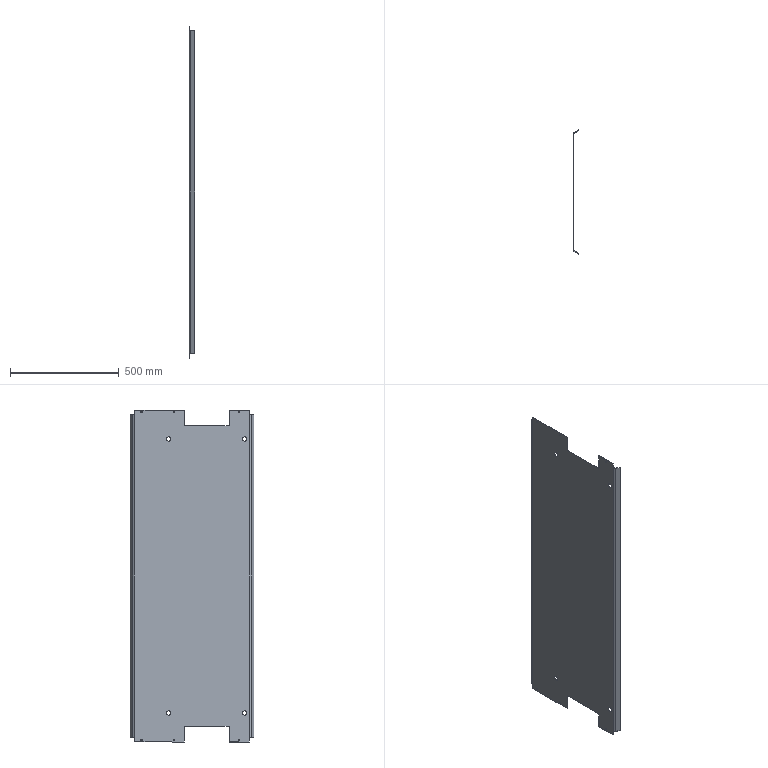Part | SolidWorks | features ICE 3, EdgeFlange 2, MirrorPattern 2, FlatPattern 1, HoleWzd 1, LPattern 1, SMBaseFlange 1, SheetMetal 1 | 1 solid | 54 faces | box 26.731 x 568.268 x 1527 mm | volume 1309231 mm3 | plane 30 | cylinder 24 | commonest cylinder face diameters 6.2 x12 20 x10 23 x2